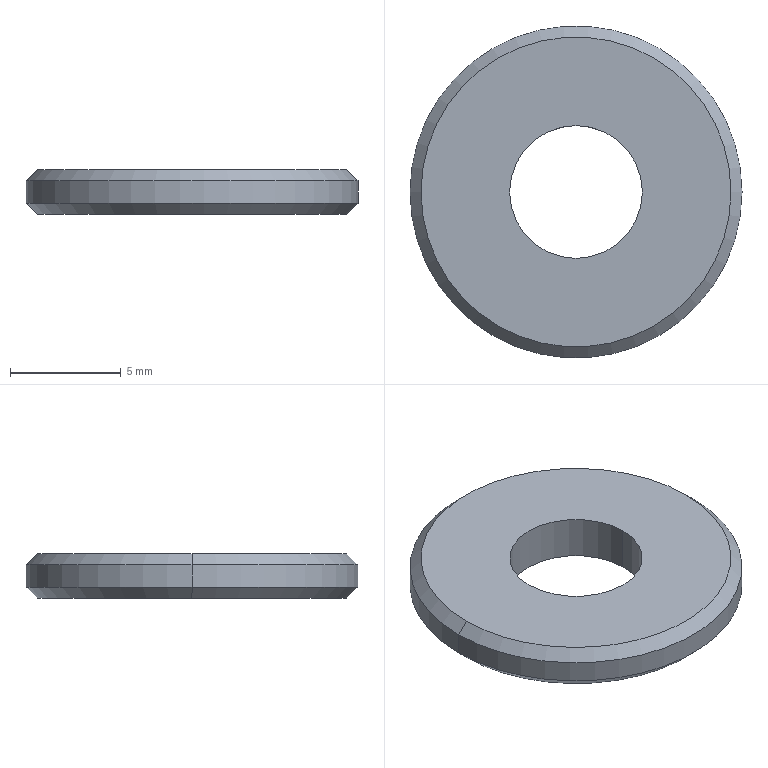Part | SolidWorks | features Attribute 3, Chamfer 1, Extrusion 1 | 1 solid | 10 faces | box 15 x 15 x 2 mm | volume 285.361 mm3 | cone 4 | cylinder 4 | plane 2 | commonest cylinder face diameters 6 x2 15 x2
STEP:
#1=CARTESIAN_POINT('',(7.,0.,2.));
#2=VERTEX_POINT('',#1);
#3=CARTESIAN_POINT('',(-7.,0.,2.));
#4=VERTEX_POINT('',#3);
#5=CARTESIAN_POINT('',(0.,0.,2.));
#6=DIRECTION('',(0.,0.,1.));
#7=DIRECTION('',(1.,0.,0.));
#8=AXIS2_PLACEMENT_3D('',#5,#6,#7);
#9=CIRCLE('',#8,7.);
#10=EDGE_CURVE('',#2,#4,#9,.T.);
#11=ORIENTED_EDGE('',*,*,#10,.F.);
#12=CARTESIAN_POINT('',(7.5,0.,1.5));
#13=VERTEX_POINT('',#12);
#14=CARTESIAN_POINT('',(7.,0.,2.));
#15=DIRECTION('',(0.7071,0.,-0.7071));
#16=VECTOR('',#15,1000.);
#17=LINE('',#14,#16);
#18=EDGE_CURVE('',#2,#13,#17,.T.);
#19=ORIENTED_EDGE('',*,*,#18,.T.);
#20=CARTESIAN_POINT('',(-7.5,0.,1.5));
#21=VERTEX_POINT('',#20);
#22=CARTESIAN_POINT('',(0.,0.,1.5));
#23=DIRECTION('',(0.,0.,-1.));
#24=DIRECTION('',(1.,0.,0.));
#25=AXIS2_PLACEMENT_3D('',#22,#23,#24);
#26=CIRCLE('',#25,7.5);
#27=EDGE_CURVE('',#21,#13,#26,.T.);
#28=ORIENTED_EDGE('',*,*,#27,.F.);
#29=CARTESIAN_POINT('',(-7.,0.,2.));
#30=DIRECTION('',(-0.7071,0.,-0.7071));
#31=VECTOR('',#30,1000.);
#32=LINE('',#29,#31);
#33=EDGE_CURVE('',#4,#21,#32,.T.);
#34=ORIENTED_EDGE('',*,*,#33,.F.);
#35=EDGE_LOOP('',(#11,#19,#28,#34));
#36=FACE_OUTER_BOUND('',#35,.T.);
#37=CARTESIAN_POINT('',(0.,0.,2.));
#38=DIRECTION('',(0.,0.,-1.));
#39=DIRECTION('',(-1.,0.,0.));
#40=AXIS2_PLACEMENT_3D('',#37,#38,#39);
#41=CONICAL_SURFACE('',#40,7.,0.7854);
#42=ADVANCED_FACE('',(#36),#41,.T.);
#43=CARTESIAN_POINT('',(-7.,0.,0.));
#44=VERTEX_POINT('',#43);
#45=CARTESIAN_POINT('',(7.,0.,0.));
#46=VERTEX_POINT('',#45);
#47=CARTESIAN_POINT('',(0.,0.,0.));
#48=DIRECTION('',(0.,0.,-1.));
#49=DIRECTION('',(1.,0.,0.));
#50=AXIS2_PLACEMENT_3D('',#47,#48,#49);
#51=CIRCLE('',#50,7.);
#52=EDGE_CURVE('',#44,#46,#51,.T.);
#53=ORIENTED_EDGE('',*,*,#52,.F.);
#54=CARTESIAN_POINT('',(-7.5,0.,0.5));
#55=VERTEX_POINT('',#54);
#56=CARTESIAN_POINT('',(-7.5,0.,0.5));
#57=DIRECTION('',(-0.7071,0.,0.7071));
#58=VECTOR('',#57,1000.);
#59=LINE('',#56,#58);
#60=EDGE_CURVE('',#44,#55,#59,.T.);
#61=ORIENTED_EDGE('',*,*,#60,.T.);
#62=CARTESIAN_POINT('',(7.5,0.,0.5));
#63=VERTEX_POINT('',#62);
#64=CARTESIAN_POINT('',(0.,0.,0.5));
#65=DIRECTION('',(0.,0.,1.));
#66=DIRECTION('',(1.,0.,0.));
#67=AXIS2_PLACEMENT_3D('',#64,#65,#66);
#68=CIRCLE('',#67,7.5);
#69=EDGE_CURVE('',#63,#55,#68,.T.);
#70=ORIENTED_EDGE('',*,*,#69,.F.);
#71=CARTESIAN_POINT('',(7.5,0.,0.5));
#72=DIRECTION('',(0.7071,0.,0.7071));
#73=VECTOR('',#72,1000.);
#74=LINE('',#71,#73);
#75=EDGE_CURVE('',#46,#63,#74,.T.);
#76=ORIENTED_EDGE('',*,*,#75,.F.);
#77=EDGE_LOOP('',(#53,#61,#70,#76));
#78=FACE_OUTER_BOUND('',#77,.T.);
#79=CARTESIAN_POINT('',(0.,0.,0.5));
#80=DIRECTION('',(0.,0.,1.));
#81=DIRECTION('',(1.,0.,0.));
#82=AXIS2_PLACEMENT_3D('',#79,#80,#81);
#83=CONICAL_SURFACE('',#82,7.5,0.7854);
#84=ADVANCED_FACE('',(#78),#83,.T.);
#85=CARTESIAN_POINT('',(-3.,0.,2.));
#86=VERTEX_POINT('',#85);
#87=CARTESIAN_POINT('',(3.,0.,2.));
#88=VERTEX_POINT('',#87);
#89=CARTESIAN_POINT('',(0.,0.,2.));
#90=DIRECTION('',(0.,0.,1.));
#91=DIRECTION('',(1.,0.,0.));
#92=AXIS2_PLACEMENT_3D('',#89,#90,#91);
#93=CIRCLE('',#92,3.);
#94=EDGE_CURVE('',#86,#88,#93,.T.);
#95=ORIENTED_EDGE('',*,*,#94,.T.);
#96=CARTESIAN_POINT('',(3.,0.,0.));
#97=VERTEX_POINT('',#96);
#98=CARTESIAN_POINT('',(3.,0.,2.));
#99=DIRECTION('',(0.,0.,-1.));
#100=VECTOR('',#99,1000.);
#101=LINE('',#98,#100);
#102=EDGE_CURVE('',#88,#97,#101,.T.);
#103=ORIENTED_EDGE('',*,*,#102,.T.);
#104=CARTESIAN_POINT('',(-3.,0.,0.));
#105=VERTEX_POINT('',#104);
#106=CARTESIAN_POINT('',(0.,0.,0.));
#107=DIRECTION('',(0.,0.,1.));
#108=DIRECTION('',(1.,0.,0.));
#109=AXIS2_PLACEMENT_3D('',#106,#107,#108);
#110=CIRCLE('',#109,3.);
#111=EDGE_CURVE('',#105,#97,#110,.T.);
#112=ORIENTED_EDGE('',*,*,#111,.F.);
#113=CARTESIAN_POINT('',(-3.,0.,2.));
#114=DIRECTION('',(0.,0.,-1.));
#115=VECTOR('',#114,1000.);
#116=LINE('',#113,#115);
#117=EDGE_CURVE('',#86,#105,#116,.T.);
#118=ORIENTED_EDGE('',*,*,#117,.F.);
#119=EDGE_LOOP('',(#95,#103,#112,#118));
#120=FACE_OUTER_BOUND('',#119,.T.);
#121=CARTESIAN_POINT('',(0.,0.,2.));
#122=DIRECTION('',(0.,0.,-1.));
#123=DIRECTION('',(-1.,0.,0.));
#124=AXIS2_PLACEMENT_3D('',#121,#122,#123);
#125=CYLINDRICAL_SURFACE('',#124,3.);
#126=ADVANCED_FACE('',(#120),#125,.F.);
#127=ORIENTED_EDGE('',*,*,#27,.T.);
#128=CARTESIAN_POINT('',(7.5,0.,2.));
#129=DIRECTION('',(0.,0.,-1.));
#130=VECTOR('',#129,1000.);
#131=LINE('',#128,#130);
#132=EDGE_CURVE('',#13,#63,#131,.T.);
#133=ORIENTED_EDGE('',*,*,#132,.T.);
#134=ORIENTED_EDGE('',*,*,#69,.T.);
#135=CARTESIAN_POINT('',(-7.5,0.,2.));
#136=DIRECTION('',(0.,0.,-1.));
#137=VECTOR('',#136,1000.);
#138=LINE('',#135,#137);
#139=EDGE_CURVE('',#21,#55,#138,.T.);
#140=ORIENTED_EDGE('',*,*,#139,.F.);
#141=EDGE_LOOP('',(#127,#133,#134,#140));
#142=FACE_OUTER_BOUND('',#141,.T.);
#143=CARTESIAN_POINT('',(0.,0.,2.));
#144=DIRECTION('',(0.,0.,-1.));
#145=DIRECTION('',(-1.,0.,0.));
#146=AXIS2_PLACEMENT_3D('',#143,#144,#145);
#147=CYLINDRICAL_SURFACE('',#146,7.5);
#148=ADVANCED_FACE('',(#142),#147,.T.);
#149=CARTESIAN_POINT('',(0.,0.,2.));
#150=DIRECTION('',(0.,0.,1.));
#151=DIRECTION('',(1.,0.,0.));
#152=AXIS2_PLACEMENT_3D('',#149,#150,#151);
#153=CIRCLE('',#152,7.);
#154=EDGE_CURVE('',#4,#2,#153,.T.);
#155=ORIENTED_EDGE('',*,*,#154,.T.);
#156=ORIENTED_EDGE('',*,*,#10,.T.);
#157=EDGE_LOOP('',(#155,#156));
#158=FACE_OUTER_BOUND('',#157,.T.);
#159=ORIENTED_EDGE('',*,*,#94,.F.);
#160=CARTESIAN_POINT('',(0.,0.,2.));
#161=DIRECTION('',(0.,0.,1.));
#162=DIRECTION('',(1.,0.,0.));
#163=AXIS2_PLACEMENT_3D('',#160,#161,#162);
#164=CIRCLE('',#163,3.);
#165=EDGE_CURVE('',#88,#86,#164,.T.);
#166=ORIENTED_EDGE('',*,*,#165,.F.);
#167=EDGE_LOOP('',(#159,#166));
#168=FACE_BOUND('',#167,.T.);
#169=CARTESIAN_POINT('',(0.,0.,2.));
#170=DIRECTION('',(0.,0.,1.));
#171=DIRECTION('',(1.,0.,0.));
#172=AXIS2_PLACEMENT_3D('',#169,#170,#171);
#173=PLANE('',#172);
#174=ADVANCED_FACE('',(#158,#168),#173,.T.);
#175=CARTESIAN_POINT('',(0.,0.,0.));
#176=DIRECTION('',(0.,0.,-1.));
#177=DIRECTION('',(1.,0.,0.));
#178=AXIS2_PLACEMENT_3D('',#175,#176,#177);
#179=CIRCLE('',#178,7.);
#180=EDGE_CURVE('',#46,#44,#179,.T.);
#181=ORIENTED_EDGE('',*,*,#180,.T.);
#182=ORIENTED_EDGE('',*,*,#52,.T.);
#183=EDGE_LOOP('',(#181,#182));
#184=FACE_OUTER_BOUND('',#183,.T.);
#185=ORIENTED_EDGE('',*,*,#111,.T.);
#186=CARTESIAN_POINT('',(0.,0.,0.));
#187=DIRECTION('',(0.,0.,1.));
#188=DIRECTION('',(1.,0.,0.));
#189=AXIS2_PLACEMENT_3D('',#186,#187,#188);
#190=CIRCLE('',#189,3.);
#191=EDGE_CURVE('',#97,#105,#190,.T.);
#192=ORIENTED_EDGE('',*,*,#191,.T.);
#193=EDGE_LOOP('',(#185,#192));
#194=FACE_BOUND('',#193,.T.);
#195=CARTESIAN_POINT('',(0.,0.,0.));
#196=DIRECTION('',(0.,0.,1.));
#197=DIRECTION('',(1.,0.,0.));
#198=AXIS2_PLACEMENT_3D('',#195,#196,#197);
#199=PLANE('',#198);
#200=ADVANCED_FACE('',(#184,#194),#199,.F.);
#201=ORIENTED_EDGE('',*,*,#132,.F.);
#202=CARTESIAN_POINT('',(0.,0.,1.5));
#203=DIRECTION('',(0.,0.,-1.));
#204=DIRECTION('',(1.,0.,0.));
#205=AXIS2_PLACEMENT_3D('',#202,#203,#204);
#206=CIRCLE('',#205,7.5);
#207=EDGE_CURVE('',#13,#21,#206,.T.);
#208=ORIENTED_EDGE('',*,*,#207,.T.);
#209=ORIENTED_EDGE('',*,*,#139,.T.);
#210=CARTESIAN_POINT('',(0.,0.,0.5));
#211=DIRECTION('',(0.,0.,1.));
#212=DIRECTION('',(1.,0.,0.));
#213=AXIS2_PLACEMENT_3D('',#210,#211,#212);
#214=CIRCLE('',#213,7.5);
#215=EDGE_CURVE('',#55,#63,#214,.T.);
#216=ORIENTED_EDGE('',*,*,#215,.T.);
#217=EDGE_LOOP('',(#201,#208,#209,#216));
#218=FACE_OUTER_BOUND('',#217,.T.);
#219=CARTESIAN_POINT('',(0.,0.,2.));
#220=DIRECTION('',(0.,0.,-1.));
#221=DIRECTION('',(-1.,0.,0.));
#222=AXIS2_PLACEMENT_3D('',#219,#220,#221);
#223=CYLINDRICAL_SURFACE('',#222,7.5);
#224=ADVANCED_FACE('',(#218),#223,.T.);
#225=ORIENTED_EDGE('',*,*,#102,.F.);
#226=ORIENTED_EDGE('',*,*,#165,.T.);
#227=ORIENTED_EDGE('',*,*,#117,.T.);
#228=ORIENTED_EDGE('',*,*,#191,.F.);
#229=EDGE_LOOP('',(#225,#226,#227,#228));
#230=FACE_OUTER_BOUND('',#229,.T.);
#231=CARTESIAN_POINT('',(0.,0.,2.));
#232=DIRECTION('',(0.,0.,-1.));
#233=DIRECTION('',(-1.,0.,0.));
#234=AXIS2_PLACEMENT_3D('',#231,#232,#233);
#235=CYLINDRICAL_SURFACE('',#234,3.);
#236=ADVANCED_FACE('',(#230),#235,.F.);
#237=ORIENTED_EDGE('',*,*,#60,.F.);
#238=ORIENTED_EDGE('',*,*,#180,.F.);
#239=ORIENTED_EDGE('',*,*,#75,.T.);
#240=ORIENTED_EDGE('',*,*,#215,.F.);
#241=EDGE_LOOP('',(#237,#238,#239,#240));
#242=FACE_OUTER_BOUND('',#241,.T.);
#243=CARTESIAN_POINT('',(0.,0.,0.5));
#244=DIRECTION('',(0.,0.,1.));
#245=DIRECTION('',(1.,0.,0.));
#246=AXIS2_PLACEMENT_3D('',#243,#244,#245);
#247=CONICAL_SURFACE('',#246,7.5,0.7854);
#248=ADVANCED_FACE('',(#242),#247,.T.);
#249=ORIENTED_EDGE('',*,*,#18,.F.);
#250=ORIENTED_EDGE('',*,*,#154,.F.);
#251=ORIENTED_EDGE('',*,*,#33,.T.);
#252=ORIENTED_EDGE('',*,*,#207,.F.);
#253=EDGE_LOOP('',(#249,#250,#251,#252));
#254=FACE_OUTER_BOUND('',#253,.T.);
#255=CARTESIAN_POINT('',(0.,0.,2.));
#256=DIRECTION('',(0.,0.,-1.));
#257=DIRECTION('',(-1.,0.,0.));
#258=AXIS2_PLACEMENT_3D('',#255,#256,#257);
#259=CONICAL_SURFACE('',#258,7.,0.7854);
#260=ADVANCED_FACE('',(#254),#259,.T.);
#261=CLOSED_SHELL('',(#42,#84,#126,#148,#174,#200,#224,#236,#248,#260));
#262=MANIFOLD_SOLID_BREP('',#261);
#263=CARTESIAN_POINT('',(0.,0.,0.));
#264=DIRECTION('',(0.,0.,1.));
#265=DIRECTION('',(1.,0.,0.));
#266=AXIS2_PLACEMENT_3D('',#263,#264,#265);
#267=(LENGTH_UNIT()NAMED_UNIT(*)SI_UNIT(.MILLI.,.METRE.));
#268=UNCERTAINTY_MEASURE_WITH_UNIT(LENGTH_MEASURE(0.00001),#267,'','');
#269=(NAMED_UNIT(*)PLANE_ANGLE_UNIT()SI_UNIT($,.RADIAN.));
#270=(NAMED_UNIT(*)SI_UNIT($,.STERADIAN.)SOLID_ANGLE_UNIT());
#271=(GEOMETRIC_REPRESENTATION_CONTEXT(3)GLOBAL_UNCERTAINTY_ASSIGNED_CONTEXT((#268))GLOBAL_UNIT_ASSIGNED_CONTEXT((#267,#269,#270))REPRESENTATION_CONTEXT('',''));
#272=ADVANCED_BREP_SHAPE_REPRESENTATION('',(#262,#266),#271);